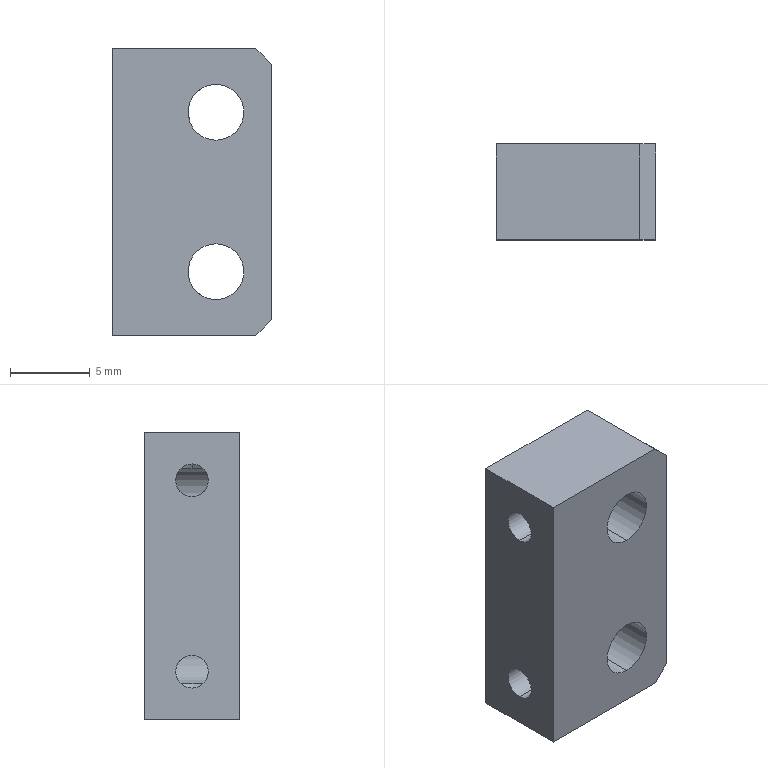Part | SolidWorks | features 3DProfileFeature 1, Chamfer 1, Extrusion 1, HoleWzd 1, ICE 1 | 1 solid | 19 faces | box 10 x 6 x 18 mm | volume 923.956 mm3 | cylinder 8 | plane 8 | cone 3 | commonest cylinder face diameters 2.05 x4 3.5 x4
STEP:
#1=CARTESIAN_POINT('',(1.35,3.,-7.025));
#2=VERTEX_POINT('',#1);
#3=CARTESIAN_POINT('',(1.35,2.294,-6.744));
#4=VERTEX_POINT('',#3);
#5=CARTESIAN_POINT('',(1.35,3.,-6.));
#6=DIRECTION('',(-1.,0.,0.));
#7=DIRECTION('',(0.,0.,1.));
#8=AXIS2_PLACEMENT_3D('',#5,#6,#7);
#9=CIRCLE('',#8,1.025);
#10=EDGE_CURVE('',#2,#4,#9,.T.);
#11=ORIENTED_EDGE('',*,*,#10,.F.);
#12=CARTESIAN_POINT('',(-5.,3.,-7.025));
#13=VERTEX_POINT('',#12);
#14=CARTESIAN_POINT('',(-5.,3.,-7.025));
#15=DIRECTION('',(-1.,0.,0.));
#16=VECTOR('',#15,1000.);
#17=LINE('',#14,#16);
#18=EDGE_CURVE('',#2,#13,#17,.T.);
#19=ORIENTED_EDGE('',*,*,#18,.T.);
#20=CARTESIAN_POINT('',(-5.,3.,-4.975));
#21=VERTEX_POINT('',#20);
#22=CARTESIAN_POINT('',(-5.,3.,-6.));
#23=DIRECTION('',(-1.,0.,0.));
#24=DIRECTION('',(0.,0.,1.));
#25=AXIS2_PLACEMENT_3D('',#22,#23,#24);
#26=CIRCLE('',#25,1.025);
#27=EDGE_CURVE('',#13,#21,#26,.T.);
#28=ORIENTED_EDGE('',*,*,#27,.T.);
#29=CARTESIAN_POINT('',(-0.2498,3.,-4.975));
#30=VERTEX_POINT('',#29);
#31=CARTESIAN_POINT('',(-5.,3.,-4.975));
#32=DIRECTION('',(-1.,0.,0.));
#33=VECTOR('',#32,1000.);
#34=LINE('',#31,#33);
#35=EDGE_CURVE('',#30,#21,#34,.T.);
#36=ORIENTED_EDGE('',*,*,#35,.F.);
#37=CARTESIAN_POINT('',(1.35,2.294,-6.744));
#38=CARTESIAN_POINT('',(1.215,2.282,-6.732));
#39=CARTESIAN_POINT('',(1.086,2.254,-6.705));
#40=CARTESIAN_POINT('',(0.8379,2.186,-6.625));
#41=CARTESIAN_POINT('',(0.719,2.146,-6.571));
#42=CARTESIAN_POINT('',(0.4974,2.071,-6.44));
#43=CARTESIAN_POINT('',(0.3923,2.036,-6.361));
#44=CARTESIAN_POINT('',(0.1992,1.986,-6.178));
#45=CARTESIAN_POINT('',(0.112,1.971,-6.074));
#46=CARTESIAN_POINT('',(-0.03695,1.98,-5.848));
#47=CARTESIAN_POINT('',(-0.09741,2.004,-5.726));
#48=CARTESIAN_POINT('',(-0.1847,2.102,-5.49));
#49=CARTESIAN_POINT('',(-0.2119,2.176,-5.376));
#50=CARTESIAN_POINT('',(-0.2429,2.364,-5.185));
#51=CARTESIAN_POINT('',(-0.2475,2.479,-5.107));
#52=CARTESIAN_POINT('',(-0.2508,2.729,-5.002));
#53=CARTESIAN_POINT('',(-0.2498,2.863,-4.975));
#54=CARTESIAN_POINT('',(-0.2498,3.,-4.975));
#55=B_SPLINE_CURVE_WITH_KNOTS('',3,(#37,#38,#39,#40,#41,#42,#43,#44,#45,#46,#47,#48,#49,#50,#51,#52,#53,#54),.UNSPECIFIED.,.F.,.F.,(4,2,2,2,2,2,2,2,4),(0.,0.0004025,0.000805,0.001207,0.00161,0.002012,0.002415,0.002817,0.00322),.UNSPECIFIED.);
#56=EDGE_CURVE('',#4,#30,#55,.T.);
#57=ORIENTED_EDGE('',*,*,#56,.F.);
#58=EDGE_LOOP('',(#11,#19,#28,#36,#57));
#59=FACE_OUTER_BOUND('',#58,.T.);
#60=CARTESIAN_POINT('',(-5.,3.,-6.));
#61=DIRECTION('',(-1.,0.,0.));
#62=DIRECTION('',(0.,0.,1.));
#63=AXIS2_PLACEMENT_3D('',#60,#61,#62);
#64=CYLINDRICAL_SURFACE('',#63,1.025);
#65=ADVANCED_FACE('',(#59),#64,.F.);
#66=CARTESIAN_POINT('',(1.515,3.,6.75));
#67=VERTEX_POINT('',#66);
#68=CARTESIAN_POINT('',(1.5,3.197,6.75));
#69=VERTEX_POINT('',#68);
#70=CARTESIAN_POINT('',(1.515,3.,6.75));
#71=CARTESIAN_POINT('',(1.515,3.066,6.75));
#72=CARTESIAN_POINT('',(1.51,3.131,6.75));
#73=CARTESIAN_POINT('',(1.5,3.197,6.75));
#74=B_SPLINE_CURVE_WITH_KNOTS('',3,(#70,#71,#72,#73),.UNSPECIFIED.,.F.,.F.,(4,4),(0.0008877,0.001086),.UNSPECIFIED.);
#75=EDGE_CURVE('',#67,#69,#74,.T.);
#76=ORIENTED_EDGE('',*,*,#75,.F.);
#77=CARTESIAN_POINT('',(1.35,3.,7.025));
#78=VERTEX_POINT('',#77);
#79=CARTESIAN_POINT('',(1.35,3.,7.025));
#80=DIRECTION('',(-0.515,0.,0.8572));
#81=VECTOR('',#80,1000.);
#82=LINE('',#79,#81);
#83=EDGE_CURVE('',#67,#78,#82,.T.);
#84=ORIENTED_EDGE('',*,*,#83,.T.);
#85=CARTESIAN_POINT('',(1.35,3.706,6.744));
#86=VERTEX_POINT('',#85);
#87=CARTESIAN_POINT('',(1.35,3.,6.));
#88=DIRECTION('',(-1.,0.,0.));
#89=DIRECTION('',(0.,0.,1.));
#90=AXIS2_PLACEMENT_3D('',#87,#88,#89);
#91=CIRCLE('',#90,1.025);
#92=EDGE_CURVE('',#78,#86,#91,.T.);
#93=ORIENTED_EDGE('',*,*,#92,.T.);
#94=CARTESIAN_POINT('',(1.5,3.197,6.75));
#95=CARTESIAN_POINT('',(1.473,3.371,6.75));
#96=CARTESIAN_POINT('',(1.416,3.541,6.749));
#97=CARTESIAN_POINT('',(1.35,3.706,6.744));
#98=B_SPLINE_CURVE_WITH_KNOTS('',3,(#94,#95,#96,#97),.UNSPECIFIED.,.F.,.F.,(4,4),(0.001086,0.001615),.UNSPECIFIED.);
#99=EDGE_CURVE('',#69,#86,#98,.T.);
#100=ORIENTED_EDGE('',*,*,#99,.F.);
#101=EDGE_LOOP('',(#76,#84,#93,#100));
#102=FACE_OUTER_BOUND('',#101,.T.);
#103=CARTESIAN_POINT('',(1.35,3.,6.));
#104=DIRECTION('',(-1.,0.,0.));
#105=DIRECTION('',(0.,0.,1.));
#106=AXIS2_PLACEMENT_3D('',#103,#104,#105);
#107=CONICAL_SURFACE('',#106,1.025,1.03);
#108=ADVANCED_FACE('',(#102),#107,.F.);
#109=CARTESIAN_POINT('',(-0.2498,3.,4.975));
#110=VERTEX_POINT('',#109);
#111=CARTESIAN_POINT('',(1.35,2.294,6.744));
#112=VERTEX_POINT('',#111);
#113=CARTESIAN_POINT('',(-0.2498,3.,4.975));
#114=CARTESIAN_POINT('',(-0.2498,2.863,4.975));
#115=CARTESIAN_POINT('',(-0.2508,2.729,5.002));
#116=CARTESIAN_POINT('',(-0.2475,2.479,5.107));
#117=CARTESIAN_POINT('',(-0.2429,2.365,5.184));
#118=CARTESIAN_POINT('',(-0.2121,2.177,5.375));
#119=CARTESIAN_POINT('',(-0.1849,2.102,5.489));
#120=CARTESIAN_POINT('',(-0.09769,2.004,5.725));
#121=CARTESIAN_POINT('',(-0.03719,1.98,5.847));
#122=CARTESIAN_POINT('',(0.1866,1.967,6.188));
#123=CARTESIAN_POINT('',(0.3862,2.034,6.374));
#124=CARTESIAN_POINT('',(0.719,2.146,6.571));
#125=CARTESIAN_POINT('',(0.8382,2.186,6.625));
#126=CARTESIAN_POINT('',(1.086,2.254,6.705));
#127=CARTESIAN_POINT('',(1.214,2.282,6.732));
#128=CARTESIAN_POINT('',(1.35,2.294,6.744));
#129=B_SPLINE_CURVE_WITH_KNOTS('',3,(#113,#114,#115,#116,#117,#118,#119,#120,#121,#122,#123,#124,#125,#126,#127,#128),.UNSPECIFIED.,.F.,.F.,(4,2,2,2,2,2,2,4),(0.00322,0.003622,0.004025,0.004427,0.004829,0.005634,0.006037,0.006439),.UNSPECIFIED.);
#130=EDGE_CURVE('',#110,#112,#129,.T.);
#131=ORIENTED_EDGE('',*,*,#130,.F.);
#132=CARTESIAN_POINT('',(-5.,3.,4.975));
#133=VERTEX_POINT('',#132);
#134=CARTESIAN_POINT('',(-5.,3.,4.975));
#135=DIRECTION('',(-1.,0.,0.));
#136=VECTOR('',#135,1000.);
#137=LINE('',#134,#136);
#138=EDGE_CURVE('',#110,#133,#137,.T.);
#139=ORIENTED_EDGE('',*,*,#138,.T.);
#140=CARTESIAN_POINT('',(-5.,3.,7.025));
#141=VERTEX_POINT('',#140);
#142=CARTESIAN_POINT('',(-5.,3.,6.));
#143=DIRECTION('',(-1.,0.,0.));
#144=DIRECTION('',(0.,0.,1.));
#145=AXIS2_PLACEMENT_3D('',#142,#143,#144);
#146=CIRCLE('',#145,1.025);
#147=EDGE_CURVE('',#133,#141,#146,.T.);
#148=ORIENTED_EDGE('',*,*,#147,.T.);
#149=CARTESIAN_POINT('',(-5.,3.,7.025));
#150=DIRECTION('',(-1.,0.,0.));
#151=VECTOR('',#150,1000.);
#152=LINE('',#149,#151);
#153=EDGE_CURVE('',#78,#141,#152,.T.);
#154=ORIENTED_EDGE('',*,*,#153,.F.);
#155=CARTESIAN_POINT('',(1.35,3.,6.));
#156=DIRECTION('',(-1.,0.,0.));
#157=DIRECTION('',(0.,0.,1.));
#158=AXIS2_PLACEMENT_3D('',#155,#156,#157);
#159=CIRCLE('',#158,1.025);
#160=EDGE_CURVE('',#112,#78,#159,.T.);
#161=ORIENTED_EDGE('',*,*,#160,.F.);
#162=EDGE_LOOP('',(#131,#139,#148,#154,#161));
#163=FACE_OUTER_BOUND('',#162,.T.);
#164=CARTESIAN_POINT('',(-5.,3.,6.));
#165=DIRECTION('',(-1.,0.,0.));
#166=DIRECTION('',(0.,0.,1.));
#167=AXIS2_PLACEMENT_3D('',#164,#165,#166);
#168=CYLINDRICAL_SURFACE('',#167,1.025);
#169=ADVANCED_FACE('',(#163),#168,.F.);
#170=CARTESIAN_POINT('',(1.5,0.,3.25));
#171=VERTEX_POINT('',#170);
#172=CARTESIAN_POINT('',(1.5,0.,6.75));
#173=VERTEX_POINT('',#172);
#174=CARTESIAN_POINT('',(1.5,0.,5.));
#175=DIRECTION('',(0.,1.,0.));
#176=DIRECTION('',(0.,0.,1.));
#177=AXIS2_PLACEMENT_3D('',#174,#175,#176);
#178=CIRCLE('',#177,1.75);
#179=EDGE_CURVE('',#171,#173,#178,.T.);
#180=ORIENTED_EDGE('',*,*,#179,.F.);
#181=CARTESIAN_POINT('',(1.5,6.,3.25));
#182=VERTEX_POINT('',#181);
#183=CARTESIAN_POINT('',(1.5,-4.,3.25));
#184=DIRECTION('',(0.,1.,0.));
#185=VECTOR('',#184,1000.);
#186=LINE('',#183,#185);
#187=EDGE_CURVE('',#171,#182,#186,.T.);
#188=ORIENTED_EDGE('',*,*,#187,.T.);
#189=CARTESIAN_POINT('',(1.5,6.,6.75));
#190=VERTEX_POINT('',#189);
#191=CARTESIAN_POINT('',(1.5,6.,5.));
#192=DIRECTION('',(0.,1.,0.));
#193=DIRECTION('',(0.,0.,-1.));
#194=AXIS2_PLACEMENT_3D('',#191,#192,#193);
#195=CIRCLE('',#194,1.75);
#196=EDGE_CURVE('',#182,#190,#195,.T.);
#197=ORIENTED_EDGE('',*,*,#196,.T.);
#198=CARTESIAN_POINT('',(1.5,-4.,6.75));
#199=DIRECTION('',(0.,1.,0.));
#200=VECTOR('',#199,1000.);
#201=LINE('',#198,#200);
#202=EDGE_CURVE('',#69,#190,#201,.T.);
#203=ORIENTED_EDGE('',*,*,#202,.F.);
#204=ORIENTED_EDGE('',*,*,#99,.T.);
#205=CARTESIAN_POINT('',(1.35,3.706,6.744));
#206=CARTESIAN_POINT('',(1.215,3.718,6.732));
#207=CARTESIAN_POINT('',(1.086,3.746,6.705));
#208=CARTESIAN_POINT('',(0.8379,3.814,6.625));
#209=CARTESIAN_POINT('',(0.719,3.854,6.571));
#210=CARTESIAN_POINT('',(0.4974,3.929,6.44));
#211=CARTESIAN_POINT('',(0.3923,3.964,6.361));
#212=CARTESIAN_POINT('',(0.1992,4.014,6.178));
#213=CARTESIAN_POINT('',(0.112,4.029,6.074));
#214=CARTESIAN_POINT('',(-0.03695,4.02,5.848));
#215=CARTESIAN_POINT('',(-0.09741,3.996,5.726));
#216=CARTESIAN_POINT('',(-0.1847,3.898,5.49));
#217=CARTESIAN_POINT('',(-0.2119,3.824,5.376));
#218=CARTESIAN_POINT('',(-0.2429,3.636,5.185));
#219=CARTESIAN_POINT('',(-0.2475,3.521,5.107));
#220=CARTESIAN_POINT('',(-0.2508,3.271,5.002));
#221=CARTESIAN_POINT('',(-0.2498,3.137,4.975));
#222=CARTESIAN_POINT('',(-0.2498,3.,4.975));
#223=B_SPLINE_CURVE_WITH_KNOTS('',3,(#205,#206,#207,#208,#209,#210,#211,#212,#213,#214,#215,#216,#217,#218,#219,#220,#221,#222),.UNSPECIFIED.,.F.,.F.,(4,2,2,2,2,2,2,2,4),(0.,0.0004025,0.000805,0.001207,0.00161,0.002012,0.002415,0.002817,0.00322),.UNSPECIFIED.);
#224=EDGE_CURVE('',#86,#110,#223,.T.);
#225=ORIENTED_EDGE('',*,*,#224,.T.);
#226=ORIENTED_EDGE('',*,*,#130,.T.);
#227=CARTESIAN_POINT('',(1.5,2.803,6.75));
#228=VERTEX_POINT('',#227);
#229=CARTESIAN_POINT('',(1.35,2.294,6.744));
#230=CARTESIAN_POINT('',(1.416,2.459,6.749));
#231=CARTESIAN_POINT('',(1.473,2.627,6.75));
#232=CARTESIAN_POINT('',(1.5,2.803,6.75));
#233=B_SPLINE_CURVE_WITH_KNOTS('',3,(#229,#230,#231,#232),.UNSPECIFIED.,.F.,.F.,(4,4),(0.00016,0.0006904),.UNSPECIFIED.);
#234=EDGE_CURVE('',#112,#228,#233,.T.);
#235=ORIENTED_EDGE('',*,*,#234,.T.);
#236=CARTESIAN_POINT('',(1.5,-4.,6.75));
#237=DIRECTION('',(0.,1.,0.));
#238=VECTOR('',#237,1000.);
#239=LINE('',#236,#238);
#240=EDGE_CURVE('',#173,#228,#239,.T.);
#241=ORIENTED_EDGE('',*,*,#240,.F.);
#242=EDGE_LOOP('',(#180,#188,#197,#203,#204,#225,#226,#235,#241));
#243=FACE_OUTER_BOUND('',#242,.T.);
#244=CARTESIAN_POINT('',(1.5,-4.,5.));
#245=DIRECTION('',(0.,1.,0.));
#246=DIRECTION('',(0.,0.,1.));
#247=AXIS2_PLACEMENT_3D('',#244,#245,#246);
#248=CYLINDRICAL_SURFACE('',#247,1.75);
#249=ADVANCED_FACE('',(#243),#248,.F.);
#250=CARTESIAN_POINT('',(1.5,0.,-6.75));
#251=VERTEX_POINT('',#250);
#252=CARTESIAN_POINT('',(1.5,0.,-3.25));
#253=VERTEX_POINT('',#252);
#254=CARTESIAN_POINT('',(1.5,0.,-5.));
#255=DIRECTION('',(0.,1.,0.));
#256=DIRECTION('',(0.,0.,1.));
#257=AXIS2_PLACEMENT_3D('',#254,#255,#256);
#258=CIRCLE('',#257,1.75);
#259=EDGE_CURVE('',#251,#253,#258,.T.);
#260=ORIENTED_EDGE('',*,*,#259,.F.);
#261=CARTESIAN_POINT('',(1.5,2.803,-6.75));
#262=VERTEX_POINT('',#261);
#263=CARTESIAN_POINT('',(1.5,-4.,-6.75));
#264=DIRECTION('',(0.,1.,0.));
#265=VECTOR('',#264,1000.);
#266=LINE('',#263,#265);
#267=EDGE_CURVE('',#251,#262,#266,.T.);
#268=ORIENTED_EDGE('',*,*,#267,.T.);
#269=CARTESIAN_POINT('',(1.5,2.803,-6.75));
#270=CARTESIAN_POINT('',(1.473,2.629,-6.75));
#271=CARTESIAN_POINT('',(1.416,2.459,-6.749));
#272=CARTESIAN_POINT('',(1.35,2.294,-6.744));
#273=B_SPLINE_CURVE_WITH_KNOTS('',3,(#269,#270,#271,#272),.UNSPECIFIED.,.F.,.F.,(4,4),(0.001086,0.001615),.UNSPECIFIED.);
#274=EDGE_CURVE('',#262,#4,#273,.T.);
#275=ORIENTED_EDGE('',*,*,#274,.T.);
#276=ORIENTED_EDGE('',*,*,#56,.T.);
#277=CARTESIAN_POINT('',(1.35,3.706,-6.744));
#278=VERTEX_POINT('',#277);
#279=CARTESIAN_POINT('',(-0.2498,3.,-4.975));
#280=CARTESIAN_POINT('',(-0.2498,3.137,-4.975));
#281=CARTESIAN_POINT('',(-0.2508,3.271,-5.002));
#282=CARTESIAN_POINT('',(-0.2475,3.521,-5.107));
#283=CARTESIAN_POINT('',(-0.2429,3.635,-5.184));
#284=CARTESIAN_POINT('',(-0.2121,3.823,-5.375));
#285=CARTESIAN_POINT('',(-0.1849,3.898,-5.489));
#286=CARTESIAN_POINT('',(-0.09769,3.996,-5.725));
#287=CARTESIAN_POINT('',(-0.03719,4.02,-5.847));
#288=CARTESIAN_POINT('',(0.1866,4.033,-6.188));
#289=CARTESIAN_POINT('',(0.3862,3.966,-6.374));
#290=CARTESIAN_POINT('',(0.719,3.854,-6.571));
#291=CARTESIAN_POINT('',(0.8382,3.814,-6.625));
#292=CARTESIAN_POINT('',(1.086,3.746,-6.705));
#293=CARTESIAN_POINT('',(1.214,3.718,-6.732));
#294=CARTESIAN_POINT('',(1.35,3.706,-6.744));
#295=B_SPLINE_CURVE_WITH_KNOTS('',3,(#279,#280,#281,#282,#283,#284,#285,#286,#287,#288,#289,#290,#291,#292,#293,#294),.UNSPECIFIED.,.F.,.F.,(4,2,2,2,2,2,2,4),(0.00322,0.003622,0.004025,0.004427,0.004829,0.005634,0.006037,0.006439),.UNSPECIFIED.);
#296=EDGE_CURVE('',#30,#278,#295,.T.);
#297=ORIENTED_EDGE('',*,*,#296,.T.);
#298=CARTESIAN_POINT('',(1.5,3.197,-6.75));
#299=VERTEX_POINT('',#298);
#300=CARTESIAN_POINT('',(1.35,3.706,-6.744));
#301=CARTESIAN_POINT('',(1.416,3.541,-6.749));
#302=CARTESIAN_POINT('',(1.473,3.373,-6.75));
#303=CARTESIAN_POINT('',(1.5,3.197,-6.75));
#304=B_SPLINE_CURVE_WITH_KNOTS('',3,(#300,#301,#302,#303),.UNSPECIFIED.,.F.,.F.,(4,4),(0.00016,0.0006904),.UNSPECIFIED.);
#305=EDGE_CURVE('',#278,#299,#304,.T.);
#306=ORIENTED_EDGE('',*,*,#305,.T.);
#307=CARTESIAN_POINT('',(1.5,6.,-6.75));
#308=VERTEX_POINT('',#307);
#309=CARTESIAN_POINT('',(1.5,-4.,-6.75));
#310=DIRECTION('',(0.,1.,0.));
#311=VECTOR('',#310,1000.);
#312=LINE('',#309,#311);
#313=EDGE_CURVE('',#299,#308,#312,.T.);
#314=ORIENTED_EDGE('',*,*,#313,.T.);
#315=CARTESIAN_POINT('',(1.5,6.,-3.25));
#316=VERTEX_POINT('',#315);
#317=CARTESIAN_POINT('',(1.5,6.,-5.));
#318=DIRECTION('',(0.,1.,0.));
#319=DIRECTION('',(0.,0.,1.));
#320=AXIS2_PLACEMENT_3D('',#317,#318,#319);
#321=CIRCLE('',#320,1.75);
#322=EDGE_CURVE('',#308,#316,#321,.T.);
#323=ORIENTED_EDGE('',*,*,#322,.T.);
#324=CARTESIAN_POINT('',(1.5,-4.,-3.25));
#325=DIRECTION('',(0.,1.,0.));
#326=VECTOR('',#325,1000.);
#327=LINE('',#324,#326);
#328=EDGE_CURVE('',#253,#316,#327,.T.);
#329=ORIENTED_EDGE('',*,*,#328,.F.);
#330=EDGE_LOOP('',(#260,#268,#275,#276,#297,#306,#314,#323,#329));
#331=FACE_OUTER_BOUND('',#330,.T.);
#332=CARTESIAN_POINT('',(1.5,-4.,-5.));
#333=DIRECTION('',(0.,1.,0.));
#334=DIRECTION('',(0.,0.,1.));
#335=AXIS2_PLACEMENT_3D('',#332,#333,#334);
#336=CYLINDRICAL_SURFACE('',#335,1.75);
#337=ADVANCED_FACE('',(#331),#336,.F.);
#338=CARTESIAN_POINT('',(5.,6.,8.));
#339=VERTEX_POINT('',#338);
#340=CARTESIAN_POINT('',(5.,6.,-8.));
#341=VERTEX_POINT('',#340);
#342=CARTESIAN_POINT('',(5.,6.,-9.));
#343=DIRECTION('',(0.,0.,-1.));
#344=VECTOR('',#343,1000.);
#345=LINE('',#342,#344);
#346=EDGE_CURVE('',#339,#341,#345,.T.);
#347=ORIENTED_EDGE('',*,*,#346,.F.);
#348=CARTESIAN_POINT('',(5.,0.,8.));
#349=VERTEX_POINT('',#348);
#350=CARTESIAN_POINT('',(5.,6.,8.));
#351=DIRECTION('',(0.,-1.,0.));
#352=VECTOR('',#351,1000.);
#353=LINE('',#350,#352);
#354=EDGE_CURVE('',#339,#349,#353,.T.);
#355=ORIENTED_EDGE('',*,*,#354,.T.);
#356=CARTESIAN_POINT('',(5.,0.,-8.));
#357=VERTEX_POINT('',#356);
#358=CARTESIAN_POINT('',(5.,0.,-9.));
#359=DIRECTION('',(0.,0.,-1.));
#360=VECTOR('',#359,1000.);
#361=LINE('',#358,#360);
#362=EDGE_CURVE('',#349,#357,#361,.T.);
#363=ORIENTED_EDGE('',*,*,#362,.T.);
#364=CARTESIAN_POINT('',(5.,6.,-8.));
#365=DIRECTION('',(0.,1.,0.));
#366=VECTOR('',#365,1000.);
#367=LINE('',#364,#366);
#368=EDGE_CURVE('',#357,#341,#367,.T.);
#369=ORIENTED_EDGE('',*,*,#368,.T.);
#370=EDGE_LOOP('',(#347,#355,#363,#369));
#371=FACE_OUTER_BOUND('',#370,.T.);
#372=CARTESIAN_POINT('',(5.,6.,-9.));
#373=DIRECTION('',(-1.,0.,0.));
#374=DIRECTION('',(0.,0.,1.));
#375=AXIS2_PLACEMENT_3D('',#372,#373,#374);
#376=PLANE('',#375);
#377=ADVANCED_FACE('',(#371),#376,.F.);
#378=CARTESIAN_POINT('',(4.,6.,-9.));
#379=VERTEX_POINT('',#378);
#380=CARTESIAN_POINT('',(-5.,6.,-9.));
#381=VERTEX_POINT('',#380);
#382=CARTESIAN_POINT('',(-5.,6.,-9.));
#383=DIRECTION('',(-1.,0.,0.));
#384=VECTOR('',#383,1000.);
#385=LINE('',#382,#384);
#386=EDGE_CURVE('',#379,#381,#385,.T.);
#387=ORIENTED_EDGE('',*,*,#386,.F.);
#388=CARTESIAN_POINT('',(4.,0.,-9.));
#389=VERTEX_POINT('',#388);
#390=CARTESIAN_POINT('',(4.,6.,-9.));
#391=DIRECTION('',(0.,-1.,0.));
#392=VECTOR('',#391,1000.);
#393=LINE('',#390,#392);
#394=EDGE_CURVE('',#379,#389,#393,.T.);
#395=ORIENTED_EDGE('',*,*,#394,.T.);
#396=CARTESIAN_POINT('',(-5.,0.,-9.));
#397=VERTEX_POINT('',#396);
#398=CARTESIAN_POINT('',(-5.,0.,-9.));
#399=DIRECTION('',(-1.,0.,0.));
#400=VECTOR('',#399,1000.);
#401=LINE('',#398,#400);
#402=EDGE_CURVE('',#389,#397,#401,.T.);
#403=ORIENTED_EDGE('',*,*,#402,.T.);
#404=CARTESIAN_POINT('',(-5.,6.,-9.));
#405=DIRECTION('',(0.,-1.,0.));
#406=VECTOR('',#405,1000.);
#407=LINE('',#404,#406);
#408=EDGE_CURVE('',#381,#397,#407,.T.);
#409=ORIENTED_EDGE('',*,*,#408,.F.);
#410=EDGE_LOOP('',(#387,#395,#403,#409));
#411=FACE_OUTER_BOUND('',#410,.T.);
#412=CARTESIAN_POINT('',(-5.,6.,-9.));
#413=DIRECTION('',(0.,0.,1.));
#414=DIRECTION('',(1.,0.,0.));
#415=AXIS2_PLACEMENT_3D('',#412,#413,#414);
#416=PLANE('',#415);
#417=ADVANCED_FACE('',(#411),#416,.F.);
#418=CARTESIAN_POINT('',(-5.,3.,-6.));
#419=DIRECTION('',(-1.,0.,0.));
#420=DIRECTION('',(0.,0.,1.));
#421=AXIS2_PLACEMENT_3D('',#418,#419,#420);
#422=CIRCLE('',#421,1.025);
#423=EDGE_CURVE('',#21,#13,#422,.T.);
#424=ORIENTED_EDGE('',*,*,#423,.F.);
#425=ORIENTED_EDGE('',*,*,#27,.F.);
#426=EDGE_LOOP('',(#424,#425));
#427=FACE_BOUND('',#426,.T.);
#428=CARTESIAN_POINT('',(-5.,3.,6.));
#429=DIRECTION('',(-1.,0.,0.));
#430=DIRECTION('',(0.,0.,1.));
#431=AXIS2_PLACEMENT_3D('',#428,#429,#430);
#432=CIRCLE('',#431,1.025);
#433=EDGE_CURVE('',#141,#133,#432,.T.);
#434=ORIENTED_EDGE('',*,*,#433,.F.);
#435=ORIENTED_EDGE('',*,*,#147,.F.);
#436=EDGE_LOOP('',(#434,#435));
#437=FACE_BOUND('',#436,.T.);
#438=CARTESIAN_POINT('',(-5.,0.,9.));
#439=VERTEX_POINT('',#438);
#440=CARTESIAN_POINT('',(-5.,0.,-9.));
#441=DIRECTION('',(0.,0.,1.));
#442=VECTOR('',#441,1000.);
#443=LINE('',#440,#442);
#444=EDGE_CURVE('',#397,#439,#443,.T.);
#445=ORIENTED_EDGE('',*,*,#444,.T.);
#446=CARTESIAN_POINT('',(-5.,6.,9.));
#447=VERTEX_POINT('',#446);
#448=CARTESIAN_POINT('',(-5.,6.,9.));
#449=DIRECTION('',(0.,-1.,0.));
#450=VECTOR('',#449,1000.);
#451=LINE('',#448,#450);
#452=EDGE_CURVE('',#447,#439,#451,.T.);
#453=ORIENTED_EDGE('',*,*,#452,.F.);
#454=CARTESIAN_POINT('',(-5.,6.,-9.));
#455=DIRECTION('',(0.,0.,1.));
#456=VECTOR('',#455,1000.);
#457=LINE('',#454,#456);
#458=EDGE_CURVE('',#381,#447,#457,.T.);
#459=ORIENTED_EDGE('',*,*,#458,.F.);
#460=ORIENTED_EDGE('',*,*,#408,.T.);
#461=EDGE_LOOP('',(#445,#453,#459,#460));
#462=FACE_OUTER_BOUND('',#461,.T.);
#463=CARTESIAN_POINT('',(-5.,6.,-9.));
#464=DIRECTION('',(1.,0.,0.));
#465=DIRECTION('',(0.,0.,-1.));
#466=AXIS2_PLACEMENT_3D('',#463,#464,#465);
#467=PLANE('',#466);
#468=ADVANCED_FACE('',(#427,#437,#462),#467,.F.);
#469=CARTESIAN_POINT('',(4.,0.,9.));
#470=VERTEX_POINT('',#469);
#471=CARTESIAN_POINT('',(-5.,0.,9.));
#472=DIRECTION('',(1.,0.,0.));
#473=VECTOR('',#472,1000.);
#474=LINE('',#471,#473);
#475=EDGE_CURVE('',#439,#470,#474,.T.);
#476=ORIENTED_EDGE('',*,*,#475,.T.);
#477=CARTESIAN_POINT('',(4.,6.,9.));
#478=VERTEX_POINT('',#477);
#479=CARTESIAN_POINT('',(4.,6.,9.));
#480=DIRECTION('',(0.,1.,0.));
#481=VECTOR('',#480,1000.);
#482=LINE('',#479,#481);
#483=EDGE_CURVE('',#470,#478,#482,.T.);
#484=ORIENTED_EDGE('',*,*,#483,.T.);
#485=CARTESIAN_POINT('',(-5.,6.,9.));
#486=DIRECTION('',(1.,0.,0.));
#487=VECTOR('',#486,1000.);
#488=LINE('',#485,#487);
#489=EDGE_CURVE('',#447,#478,#488,.T.);
#490=ORIENTED_EDGE('',*,*,#489,.F.);
#491=ORIENTED_EDGE('',*,*,#452,.T.);
#492=EDGE_LOOP('',(#476,#484,#490,#491));
#493=FACE_OUTER_BOUND('',#492,.T.);
#494=CARTESIAN_POINT('',(-5.,6.,9.));
#495=DIRECTION('',(0.,0.,-1.));
#496=DIRECTION('',(-1.,0.,0.));
#497=AXIS2_PLACEMENT_3D('',#494,#495,#496);
#498=PLANE('',#497);
#499=ADVANCED_FACE('',(#493),#498,.F.);
#500=CARTESIAN_POINT('',(1.5,6.,5.));
#501=DIRECTION('',(0.,1.,0.));
#502=DIRECTION('',(0.,0.,-1.));
#503=AXIS2_PLACEMENT_3D('',#500,#501,#502);
#504=CIRCLE('',#503,1.75);
#505=EDGE_CURVE('',#190,#182,#504,.T.);
#506=ORIENTED_EDGE('',*,*,#505,.F.);
#507=ORIENTED_EDGE('',*,*,#196,.F.);
#508=EDGE_LOOP('',(#506,#507));
#509=FACE_BOUND('',#508,.T.);
#510=CARTESIAN_POINT('',(1.5,6.,-5.));
#511=DIRECTION('',(0.,1.,0.));
#512=DIRECTION('',(0.,0.,1.));
#513=AXIS2_PLACEMENT_3D('',#510,#511,#512);
#514=CIRCLE('',#513,1.75);
#515=EDGE_CURVE('',#316,#308,#514,.T.);
#516=ORIENTED_EDGE('',*,*,#515,.F.);
#517=ORIENTED_EDGE('',*,*,#322,.F.);
#518=EDGE_LOOP('',(#516,#517));
#519=FACE_BOUND('',#518,.T.);
#520=ORIENTED_EDGE('',*,*,#489,.T.);
#521=CARTESIAN_POINT('',(6.5,6.,6.5));
#522=DIRECTION('',(0.7071,0.,-0.7071));
#523=VECTOR('',#522,1000.);
#524=LINE('',#521,#523);
#525=EDGE_CURVE('',#478,#339,#524,.T.);
#526=ORIENTED_EDGE('',*,*,#525,.T.);
#527=ORIENTED_EDGE('',*,*,#346,.T.);
#528=CARTESIAN_POINT('',(6.5,6.,-6.5));
#529=DIRECTION('',(-0.7071,0.,-0.7071));
#530=VECTOR('',#529,1000.);
#531=LINE('',#528,#530);
#532=EDGE_CURVE('',#341,#379,#531,.T.);
#533=ORIENTED_EDGE('',*,*,#532,.T.);
#534=ORIENTED_EDGE('',*,*,#386,.T.);
#535=ORIENTED_EDGE('',*,*,#458,.T.);
#536=EDGE_LOOP('',(#520,#526,#527,#533,#534,#535));
#537=FACE_OUTER_BOUND('',#536,.T.);
#538=CARTESIAN_POINT('',(0.,6.,0.));
#539=DIRECTION('',(0.,1.,0.));
#540=DIRECTION('',(0.,0.,1.));
#541=AXIS2_PLACEMENT_3D('',#538,#539,#540);
#542=PLANE('',#541);
#543=ADVANCED_FACE('',(#509,#519,#537),#542,.T.);
#544=CARTESIAN_POINT('',(1.5,0.,5.));
#545=DIRECTION('',(0.,1.,0.));
#546=DIRECTION('',(0.,0.,1.));
#547=AXIS2_PLACEMENT_3D('',#544,#545,#546);
#548=CIRCLE('',#547,1.75);
#549=EDGE_CURVE('',#173,#171,#548,.T.);
#550=ORIENTED_EDGE('',*,*,#549,.T.);
#551=ORIENTED_EDGE('',*,*,#179,.T.);
#552=EDGE_LOOP('',(#550,#551));
#553=FACE_BOUND('',#552,.T.);
#554=CARTESIAN_POINT('',(1.5,0.,-5.));
#555=DIRECTION('',(0.,1.,0.));
#556=DIRECTION('',(0.,0.,1.));
#557=AXIS2_PLACEMENT_3D('',#554,#555,#556);
#558=CIRCLE('',#557,1.75);
#559=EDGE_CURVE('',#253,#251,#558,.T.);
#560=ORIENTED_EDGE('',*,*,#559,.T.);
#561=ORIENTED_EDGE('',*,*,#259,.T.);
#562=EDGE_LOOP('',(#560,#561));
#563=FACE_BOUND('',#562,.T.);
#564=ORIENTED_EDGE('',*,*,#362,.F.);
#565=CARTESIAN_POINT('',(5.,0.,8.));
#566=DIRECTION('',(-0.7071,0.,0.7071));
#567=VECTOR('',#566,1000.);
#568=LINE('',#565,#567);
#569=EDGE_CURVE('',#349,#470,#568,.T.);
#570=ORIENTED_EDGE('',*,*,#569,.T.);
#571=ORIENTED_EDGE('',*,*,#475,.F.);
#572=ORIENTED_EDGE('',*,*,#444,.F.);
#573=ORIENTED_EDGE('',*,*,#402,.F.);
#574=CARTESIAN_POINT('',(4.,0.,-9.));
#575=DIRECTION('',(0.7071,0.,0.7071));
#576=VECTOR('',#575,1000.);
#577=LINE('',#574,#576);
#578=EDGE_CURVE('',#389,#357,#577,.T.);
#579=ORIENTED_EDGE('',*,*,#578,.T.);
#580=EDGE_LOOP('',(#564,#570,#571,#572,#573,#579));
#581=FACE_OUTER_BOUND('',#580,.T.);
#582=CARTESIAN_POINT('',(0.,0.,0.));
#583=DIRECTION('',(0.,1.,0.));
#584=DIRECTION('',(0.,0.,1.));
#585=AXIS2_PLACEMENT_3D('',#582,#583,#584);
#586=PLANE('',#585);
#587=ADVANCED_FACE('',(#553,#563,#581),#586,.F.);
#588=ORIENTED_EDGE('',*,*,#267,.F.);
#589=ORIENTED_EDGE('',*,*,#559,.F.);
#590=ORIENTED_EDGE('',*,*,#328,.T.);
#591=ORIENTED_EDGE('',*,*,#515,.T.);
#592=ORIENTED_EDGE('',*,*,#313,.F.);
#593=CARTESIAN_POINT('',(1.5,3.197,-6.75));
#594=CARTESIAN_POINT('',(1.52,3.065,-6.75));
#595=CARTESIAN_POINT('',(1.52,2.934,-6.75));
#596=CARTESIAN_POINT('',(1.5,2.803,-6.75));
#597=B_SPLINE_CURVE_WITH_KNOTS('',3,(#593,#594,#595,#596),.UNSPECIFIED.,.F.,.F.,(4,4),(0.0006904,0.001086),.UNSPECIFIED.);
#598=EDGE_CURVE('',#299,#262,#597,.T.);
#599=ORIENTED_EDGE('',*,*,#598,.T.);
#600=EDGE_LOOP('',(#588,#589,#590,#591,#592,#599));
#601=FACE_OUTER_BOUND('',#600,.T.);
#602=CARTESIAN_POINT('',(1.5,-4.,-5.));
#603=DIRECTION('',(0.,1.,0.));
#604=DIRECTION('',(0.,0.,1.));
#605=AXIS2_PLACEMENT_3D('',#602,#603,#604);
#606=CYLINDRICAL_SURFACE('',#605,1.75);
#607=ADVANCED_FACE('',(#601),#606,.F.);
#608=ORIENTED_EDGE('',*,*,#187,.F.);
#609=ORIENTED_EDGE('',*,*,#549,.F.);
#610=ORIENTED_EDGE('',*,*,#240,.T.);
#611=CARTESIAN_POINT('',(1.5,2.803,6.75));
#612=CARTESIAN_POINT('',(1.51,2.869,6.75));
#613=CARTESIAN_POINT('',(1.515,2.935,6.75));
#614=CARTESIAN_POINT('',(1.515,3.,6.75));
#615=B_SPLINE_CURVE_WITH_KNOTS('',3,(#611,#612,#613,#614),.UNSPECIFIED.,.F.,.F.,(4,4),(0.0006904,0.0008877),.UNSPECIFIED.);
#616=EDGE_CURVE('',#228,#67,#615,.T.);
#617=ORIENTED_EDGE('',*,*,#616,.T.);
#618=ORIENTED_EDGE('',*,*,#75,.T.);
#619=ORIENTED_EDGE('',*,*,#202,.T.);
#620=ORIENTED_EDGE('',*,*,#505,.T.);
#621=EDGE_LOOP('',(#608,#609,#610,#617,#618,#619,#620));
#622=FACE_OUTER_BOUND('',#621,.T.);
#623=CARTESIAN_POINT('',(1.5,-4.,5.));
#624=DIRECTION('',(0.,1.,0.));
#625=DIRECTION('',(0.,0.,1.));
#626=AXIS2_PLACEMENT_3D('',#623,#624,#625);
#627=CYLINDRICAL_SURFACE('',#626,1.75);
#628=ADVANCED_FACE('',(#622),#627,.F.);
#629=ORIENTED_EDGE('',*,*,#525,.F.);
#630=ORIENTED_EDGE('',*,*,#483,.F.);
#631=ORIENTED_EDGE('',*,*,#569,.F.);
#632=ORIENTED_EDGE('',*,*,#354,.F.);
#633=EDGE_LOOP('',(#629,#630,#631,#632));
#634=FACE_OUTER_BOUND('',#633,.T.);
#635=CARTESIAN_POINT('',(5.,6.,8.));
#636=DIRECTION('',(-0.7071,0.,-0.7071));
#637=DIRECTION('',(0.,-1.,0.));
#638=AXIS2_PLACEMENT_3D('',#635,#636,#637);
#639=PLANE('',#638);
#640=ADVANCED_FACE('',(#634),#639,.F.);
#641=ORIENTED_EDGE('',*,*,#532,.F.);
#642=ORIENTED_EDGE('',*,*,#368,.F.);
#643=ORIENTED_EDGE('',*,*,#578,.F.);
#644=ORIENTED_EDGE('',*,*,#394,.F.);
#645=EDGE_LOOP('',(#641,#642,#643,#644));
#646=FACE_OUTER_BOUND('',#645,.T.);
#647=CARTESIAN_POINT('',(4.,6.,-9.));
#648=DIRECTION('',(-0.7071,0.,0.7071));
#649=DIRECTION('',(0.,-1.,0.));
#650=AXIS2_PLACEMENT_3D('',#647,#648,#649);
#651=PLANE('',#650);
#652=ADVANCED_FACE('',(#646),#651,.F.);
#653=ORIENTED_EDGE('',*,*,#138,.F.);
#654=ORIENTED_EDGE('',*,*,#224,.F.);
#655=ORIENTED_EDGE('',*,*,#92,.F.);
#656=ORIENTED_EDGE('',*,*,#153,.T.);
#657=ORIENTED_EDGE('',*,*,#433,.T.);
#658=EDGE_LOOP('',(#653,#654,#655,#656,#657));
#659=FACE_OUTER_BOUND('',#658,.T.);
#660=CARTESIAN_POINT('',(-5.,3.,6.));
#661=DIRECTION('',(-1.,0.,0.));
#662=DIRECTION('',(0.,0.,1.));
#663=AXIS2_PLACEMENT_3D('',#660,#661,#662);
#664=CYLINDRICAL_SURFACE('',#663,1.025);
#665=ADVANCED_FACE('',(#659),#664,.F.);
#666=ORIENTED_EDGE('',*,*,#83,.F.);
#667=ORIENTED_EDGE('',*,*,#616,.F.);
#668=ORIENTED_EDGE('',*,*,#234,.F.);
#669=ORIENTED_EDGE('',*,*,#160,.T.);
#670=EDGE_LOOP('',(#666,#667,#668,#669));
#671=FACE_OUTER_BOUND('',#670,.T.);
#672=CARTESIAN_POINT('',(1.35,3.,6.));
#673=DIRECTION('',(-1.,0.,0.));
#674=DIRECTION('',(0.,0.,1.));
#675=AXIS2_PLACEMENT_3D('',#672,#673,#674);
#676=CONICAL_SURFACE('',#675,1.025,1.03);
#677=ADVANCED_FACE('',(#671),#676,.F.);
#678=CARTESIAN_POINT('',(1.35,3.,-6.));
#679=DIRECTION('',(-1.,0.,0.));
#680=DIRECTION('',(0.,0.,1.));
#681=AXIS2_PLACEMENT_3D('',#678,#679,#680);
#682=CIRCLE('',#681,1.025);
#683=EDGE_CURVE('',#278,#2,#682,.T.);
#684=ORIENTED_EDGE('',*,*,#683,.T.);
#685=ORIENTED_EDGE('',*,*,#10,.T.);
#686=ORIENTED_EDGE('',*,*,#274,.F.);
#687=ORIENTED_EDGE('',*,*,#598,.F.);
#688=ORIENTED_EDGE('',*,*,#305,.F.);
#689=EDGE_LOOP('',(#684,#685,#686,#687,#688));
#690=FACE_OUTER_BOUND('',#689,.T.);
#691=CARTESIAN_POINT('',(1.35,3.,-6.));
#692=DIRECTION('',(-1.,0.,0.));
#693=DIRECTION('',(0.,0.,1.));
#694=AXIS2_PLACEMENT_3D('',#691,#692,#693);
#695=CONICAL_SURFACE('',#694,1.025,1.03);
#696=ADVANCED_FACE('',(#690),#695,.F.);
#697=ORIENTED_EDGE('',*,*,#18,.F.);
#698=ORIENTED_EDGE('',*,*,#683,.F.);
#699=ORIENTED_EDGE('',*,*,#296,.F.);
#700=ORIENTED_EDGE('',*,*,#35,.T.);
#701=ORIENTED_EDGE('',*,*,#423,.T.);
#702=EDGE_LOOP('',(#697,#698,#699,#700,#701));
#703=FACE_OUTER_BOUND('',#702,.T.);
#704=CARTESIAN_POINT('',(-5.,3.,-6.));
#705=DIRECTION('',(-1.,0.,0.));
#706=DIRECTION('',(0.,0.,1.));
#707=AXIS2_PLACEMENT_3D('',#704,#705,#706);
#708=CYLINDRICAL_SURFACE('',#707,1.025);
#709=ADVANCED_FACE('',(#703),#708,.F.);
#710=CLOSED_SHELL('',(#65,#108,#169,#249,#337,#377,#417,#468,#499,#543,#587,#607,#628,#640,#652,#665,#677,#696,#709));
#711=MANIFOLD_SOLID_BREP('',#710);
#712=CARTESIAN_POINT('',(0.,0.,0.));
#713=DIRECTION('',(0.,0.,1.));
#714=DIRECTION('',(1.,0.,0.));
#715=AXIS2_PLACEMENT_3D('',#712,#713,#714);
#716=(LENGTH_UNIT()NAMED_UNIT(*)SI_UNIT(.MILLI.,.METRE.));
#717=UNCERTAINTY_MEASURE_WITH_UNIT(LENGTH_MEASURE(0.00001),#716,'','');
#718=(NAMED_UNIT(*)PLANE_ANGLE_UNIT()SI_UNIT($,.RADIAN.));
#719=(NAMED_UNIT(*)SI_UNIT($,.STERADIAN.)SOLID_ANGLE_UNIT());
#720=(GEOMETRIC_REPRESENTATION_CONTEXT(3)GLOBAL_UNCERTAINTY_ASSIGNED_CONTEXT((#717))GLOBAL_UNIT_ASSIGNED_CONTEXT((#716,#718,#719))REPRESENTATION_CONTEXT('',''));
#721=ADVANCED_BREP_SHAPE_REPRESENTATION('',(#711,#715),#720);